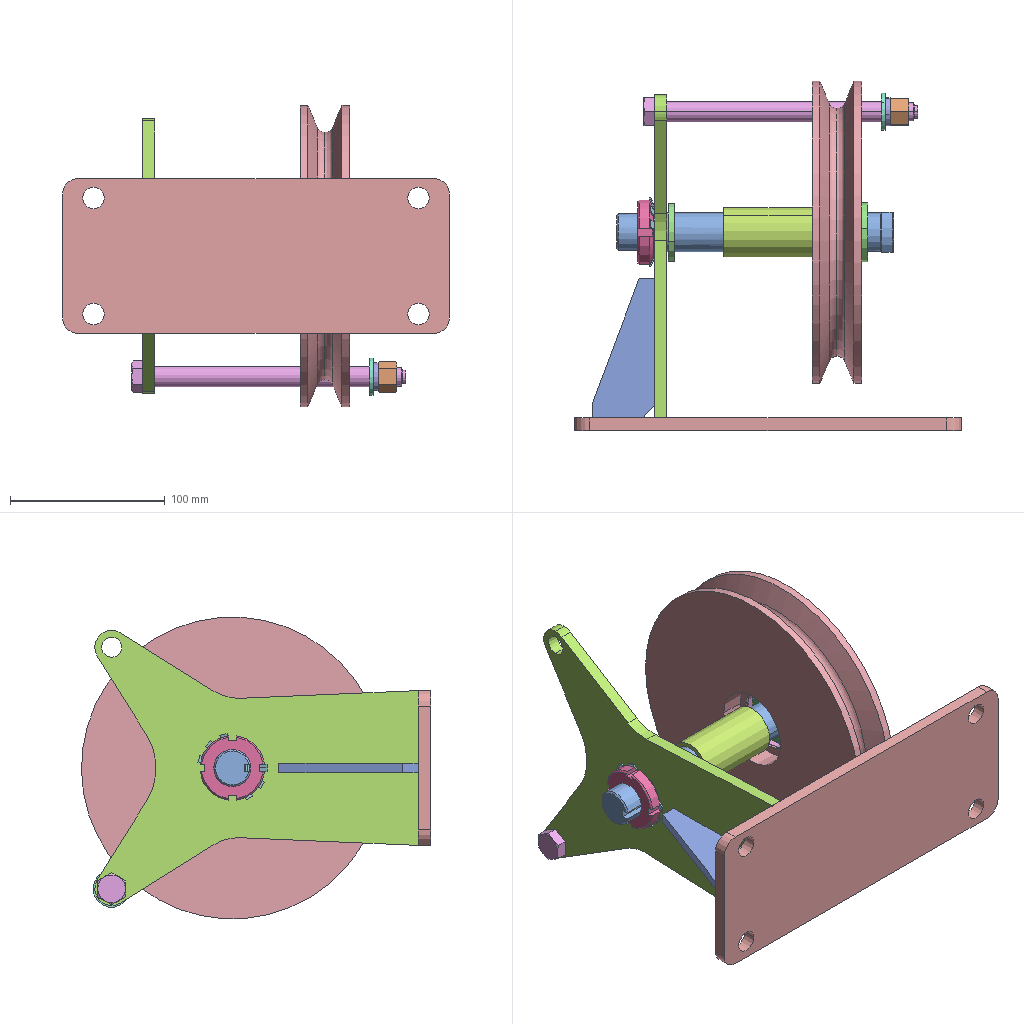Assembly | SolidWorks | 16 different items | 17 placed | box 250 x 225 x 195 mm
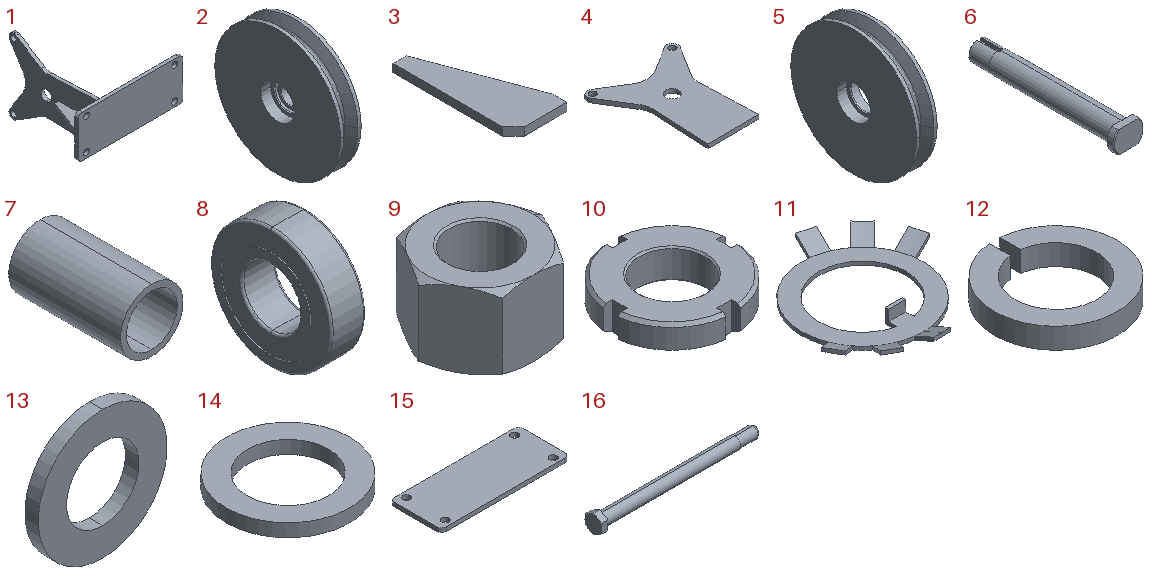Parts list (item | name | quantity | parent item | size | volume | features):
1 | (subassembly) | x1 | - | 250 x 216.909 x 177.818 mm | 364616 mm3 | -
2 | (subassembly) | x1 | - | 32 x 195 x 195 mm | 764885 mm3 | -
3 | - | x1 | in 1 | 40 x 90 x 6 mm | 14208 mm3 | features Chamfer 1, Extrusion 1
4 | - | x1 | in 1 | 177.818 x 208.909 x 8 mm | 156021 mm3 | features Extrusion 1
5 | - | x1 | in 2 | 32 x 195 x 195 mm | 746203 mm3 | features ICE 2, MirrorPattern 1, Revolution 1
6 | - | x1 | - | 36 x 179 x 26 mm | 89159 mm3 | features Chamfer 2, Fillet 2, ICE 2, Revolution 1
7 | - | x1 | - | 32 x 57 x 32 mm | 15579 mm3 | features Chamfer 1, Extrusion 1
8 | - | x1 | in 2 | 15 x 52 x 52 mm | 18682 mm3 | features Revolution 3, CirPattern 1, RefAxis 1
9 | - | x1 | - | 19.9 x 17.234 x 12.2 mm | 2145 mm3 | features Cut 2, Chamfer 1, Extrusion 1
10 | - | x1 | - | 41.701 x 41.701 x 10 mm | 8727 mm3 | features Chamfer 3, CirPattern 1, Cut 1, Extrusion 1
11 | - | x1 | - | 42.805 x 44.602 x 4 mm | 623.641 mm3 | features Boss 1, Cut 1, Revolution 1
12 | - | x1 | - | 18.367 x 18.334 x 3.1 mm | 444.091 mm3 | features Extrusion 1
13 | - | x1 | - | 24 x 2.5 x 24 mm | 773.126 mm3 | features Revolution 1
14 | - | x2 | - | 38 x 38 x 4 mm | 2573 mm3 | features Extrusion 1
15 | - | x1 | in 1 | 250 x 100 x 8 mm | 194387 mm3 | features Chamfer 1, Extrusion 1, Fillet 1, HoleWzd 1
16 | - | x1 | - | 177 x 18 x 20.785 mm | 23953 mm3 | features RevCut 2, Chamfer 1, Extrusion 1, Fillet 1, LPattern 1, MoveCopyBody 1, Revolution 1
Mates (type | each side: item.copy, entity, surface, feature):
In the top assembly
Concentric | 16.1 face cylinder Boss-Revolve1 | 13.1 face cylinder Boss-Revolve
Concentric | 16.1 face cylinder Boss-Revolve1 | 12.1 face cylinder Extrude1
Concentric | 16.1 face cylinder Boss-Revolve1 | 9.1 face cylinder Boss-Extrude
Concentric | 4.1 face cylinder Boss-Extrude1 | 16.1 face cylinder Boss-Revolve1
Coincident | 4.1 face plane Boss-Extrude1 | 16.1 face plane Boss-Extrude
Coincident | assembly face | 13.1 face plane Boss-Revolve
Coincident | 12.1 face plane Extrude1 | 13.1 face plane Boss-Revolve
Coincident | 9.1 face plane Boss-Extrude | 12.1 face plane Extrude1
Concentric | assembly face | 6.1 face cylinder Revolve1
Coincident | assembly face | 6.1 face plane Revolve1
Parallel | assembly face | 6.1 face plane Cut-Extrude1
Concentric | 5.1 face cylinder Revolve1 | 6.1 face cylinder Revolve1
Concentric | 6.1 face cylinder Revolve1 | 7.1 face cylinder Boss-Extrude1
Coincident | assembly face | 7.1 face plane Boss-Extrude1
Concentric | 5.1 face cylinder Revolve1 | 14.1 face cylinder Extrude1
Coincident | 8.1 face plane Revolve1 | 14.1 face plane Extrude1
Concentric | 6.1 face cylinder Revolve1 | 11.1 face cylinder Cut-Extrude2
Concentric | 6.1 face cylinder Revolve1 | 10.1 face cylinder Boss-Extrude
Parallel | 6.1 face plane Cut-Extrude2 | 11.1 face plane Cut-Extrude2
Coincident | 4.1 face plane Boss-Extrude1 | 11.1 face plane Boss-Revolve
Coincident | 10.1 face plane Boss-Extrude | 11.1 face plane Boss-Revolve
Coincident | 6.1 face plane Cut-Extrude2 | 10.1 face plane CirPattern1
In subassembly 1
Coincident | 15.1 face plane Boss-Extrude1 | 1.1 plane
Coincident | 15.1 plane | 1.1 plane | 2 times
Coincident | 15.1 face plane Boss-Extrude1 | 4.2 face plane Boss-Extrude1
Coincident | 15.1 edge | 4.2 face plane Boss-Extrude1
Coincident | 3.1 face plane Boss-Extrude1 | 15.1 face plane Boss-Extrude1
Coincident | 3.1 face plane Boss-Extrude1 | 4.2 face plane Boss-Extrude1
Width | 3.1 face plane Boss-Extrude1 | 3.1 face plane Boss-Extrude1 | 15.1 face plane Boss-Extrude1 | 15.1 face plane Boss-Extrude1
In subassembly 2
Concentric | 5.2 face cylinder Cut-Extrude2 | 8.2 face cylinder Revolve1
Coincident | 5.2 face plane Cut-Extrude2 | 8.2 face plane Revolve1